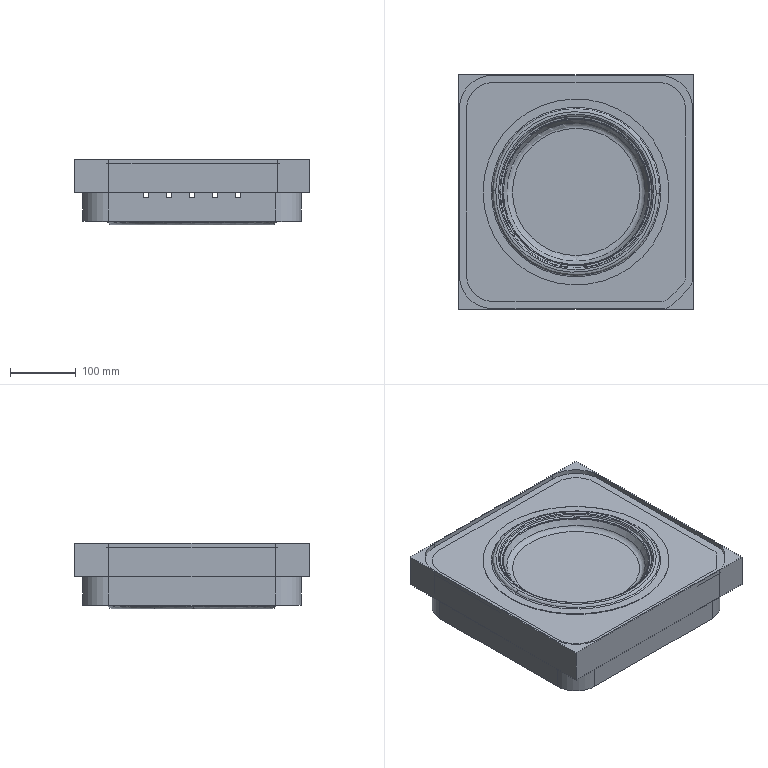NC program | NX | posted with a generic post | part box 356 x 356 x 99.5 mm
Lines 1 to 1240 of 165566:
N10 G17 G21 G94 G90
(01 , TOOL : D16R0.8)
N12 T00 M6
N14 G53
N16 G17 G0 G90 X-168.87 Y-27.35 S7000 M3 M8
N18 G43 Z200.5 H0
N20 Z51.5
N22 G94 G1 Y0. Z50.067 F4500.
N24 Y126.
N26 G2 X-126. Y168.87 R42.87
N28 G1 X126.
N30 G2 X168.87 Y126. R42.87
N32 G1 Y-129.787
N34 G2 X163.658 Y-142.401 R17.87
N36 G1 X163.609 Y-142.45
N38 X142.447 Y-163.612
N40 X142.398 Y-163.661
N42 G2 X129.787 Y-168.87 R17.87
N44 G1 X-126.
N46 G2 X-168.87 Y-126. R42.87
N48 G1 Y0.
N50 X-158.79
N52 Y126.
N54 G2 X-126. Y158.79 R32.79
N56 G1 X126.
N58 G2 X158.79 Y126. R32.79
N60 G1 Y-129.787
N62 G2 X156.48 Y-135.323 R7.79
N64 G1 X135.321 Y-156.482
N66 G2 X129.787 Y-158.79 R7.79
N68 G1 X-126.
N70 G2 X-158.79 Y-126. R32.79
N72 G1 Y0.
N74 X-148.71
N76 Y126.
N78 G2 X-126. Y148.71 R22.71
N80 G1 X126.
N82 G2 X148.71 Y126. R22.71
N84 G1 Y-128.838
N86 X128.838 Y-148.71
N88 X-126.
N90 G2 X-148.71 Y-126. R22.71
N92 G1 Y0.
N94 X-138.63
N96 Y126.
N98 G2 X-126. Y138.63 R12.63
N100 G1 X126.
N102 G2 X138.63 Y126. R12.63
N104 G1 Y-124.663
N106 X124.663 Y-138.63
N108 X-126.
N110 G2 X-138.63 Y-126. R12.63
N112 G1 Y0.
N114 X-128.55
N116 Y126.
N118 G2 X-126. Y128.55 R2.55
N120 G1 X126.
N122 G2 X128.55 Y126. R2.55
N124 G1 Y-120.488
N126 X120.488 Y-128.55
N128 X-126.
N130 G2 X-128.55 Y-126. R2.55
N132 G1 Y0.
N134 X-118.47
N136 Y118.47
N138 X118.47
N140 Y-116.312
N142 X116.312 Y-118.47
N144 X-118.47
N146 Y0.
N148 X-108.39
N150 Y108.39
N152 X108.39
N154 Y-108.39
N156 X-108.39
N158 Y0.
N160 X-98.31
N162 Y98.31
N164 X98.31
N166 Y-98.31
N168 X-98.31
N170 Y0.
N172 X-88.23
N174 Y88.23
N176 X88.23
N178 Y-88.23
N180 X-88.23
N182 Y0.
N184 X-78.15
N186 Y78.15
N188 X78.15
N190 Y-78.15
N192 X-78.15
N194 Y0.
N196 X-68.07
N198 Y68.07
N200 X68.07
N202 Y-68.07
N204 X-68.07
N206 Y0.
N208 X-57.99
N210 Y57.99
N212 X57.99
N214 Y-57.99
N216 X-57.99
N218 Y0.
N220 X-47.91
N222 Y47.91
N224 X47.91
N226 Y-47.91
N228 X-47.91
N230 Y0.
N232 X-37.83
N234 Y37.83
N236 X37.83
N238 Y-37.83
N240 X-37.83
N242 Y0.
N244 X-27.75
N246 Y27.75
N248 X27.75
N250 Y-27.75
N252 X-27.75
N254 Y0.
N256 X-17.67
N258 Y17.67
N260 X17.67
N262 Y-17.67
N264 X-17.67
N266 Y0.
N268 X-7.59
N270 Y7.59
N272 X7.59
N274 Y-7.59
N276 X-7.59
N278 Y0.
N280 X-0.39
N282 Y0.39
N284 X0.39
N286 Y-0.39
N288 X-0.39
N290 Y0.
N292 G3 X-3.59 Y3.2 R3.2
N294 G1 Z51.067
N296 G0 Z53.5
N298 X-168.8 Y-27.35
N300 Z51.067
N302 G1 Y0. Z49.633
N304 Y126.
N306 G2 X-126. Y168.8 R42.8
N308 G1 X126.
N310 G2 X168.8 Y126. R42.8
N312 G1 Y-129.787
N314 G2 X163.587 Y-142.373 R17.8
N316 G1 X142.373 Y-163.587
N318 G2 X129.787 Y-168.8 R17.8
N320 G1 X-126.
N322 G2 X-168.8 Y-126. R42.8
N324 G1 Y0.
N326 X-158.72
N328 Y126.
N330 G2 X-126. Y158.72 R32.72
N332 G1 X126.
N334 G2 X158.72 Y126. R32.72
N336 G1 Y-129.787
N338 G2 X156.459 Y-135.246 R7.72
N340 G1 X135.246 Y-156.459
N342 G2 X129.787 Y-158.72 R7.72
N344 G1 X-126.
N346 G2 X-158.72 Y-126. R32.72
N348 G1 Y0.
N350 X-148.64
N352 Y126.
N354 G2 X-126. Y148.64 R22.64
N356 G1 X126.
N358 G2 X148.64 Y126. R22.64
N360 G1 Y-128.809
N362 X128.809 Y-148.64
N364 X-126.
N366 G2 X-148.64 Y-126. R22.64
N368 G1 Y0.
N370 X-138.56
N372 Y126.
N374 G2 X-126. Y138.56 R12.56
N376 G1 X126.
N378 G2 X138.56 Y126. R12.56
N380 G1 Y-124.634
N382 X124.634 Y-138.56
N384 X-126.
N386 G2 X-138.56 Y-126. R12.56
N388 G1 Y0.
N390 X-128.48
N392 Y126.
N394 G2 X-126. Y128.48 R2.48
N396 G1 X126.
N398 G2 X128.48 Y126. R2.48
N400 G1 Y-120.459
N402 X120.459 Y-128.48
N404 X-126.
N406 G2 X-128.48 Y-126. R2.48
N408 G1 Y0.
N410 X-118.4
N412 Y118.4
N414 X118.4
N416 Y-116.283
N418 X116.283 Y-118.4
N420 X-118.4
N422 Y0.
N424 X-108.32
N426 Y108.32
N428 X108.32
N430 Y-108.32
N432 X-108.32
N434 Y0.
N436 X-98.24
N438 Y98.24
N440 X98.24
N442 Y-98.24
N444 X-98.24
N446 Y0.
N448 X-88.16
N450 Y88.16
N452 X88.16
N454 Y-88.16
N456 X-88.16
N458 Y0.
N460 X-78.08
N462 Y78.08
N464 X78.08
N466 Y-78.08
N468 X-78.08
N470 Y0.
N472 X-68.
N474 Y68.
N476 X68.
N478 Y-68.
N480 X-68.
N482 Y0.
N484 X-57.92
N486 Y57.92
N488 X57.92
N490 Y-57.92
N492 X-57.92
N494 Y0.
N496 X-47.84
N498 Y47.84
N500 X47.84
N502 Y-47.84
N504 X-47.84
N506 Y0.
N508 X-37.76
N510 Y37.76
N512 X37.76
N514 Y-37.76
N516 X-37.76
N518 Y0.
N520 X-27.68
N522 Y27.68
N524 X27.68
N526 Y-27.68
N528 X-27.68
N530 Y0.
N532 X-17.6
N534 Y17.6
N536 X17.6
N538 Y-17.6
N540 X-17.6
N542 Y0.
N544 X-7.52
N546 Y7.52
N548 X7.52
N550 Y-7.52
N552 X-7.52
N554 Y0.
N556 X-0.32
N558 Y0.32
N560 X0.32
N562 Y-0.32
N564 X-0.32
N566 Y0.
N568 G3 X-3.52 Y3.2 R3.2
N570 G1 Z50.633
N572 G0 Z53.067
N574 X-168.8 Y-27.35
N576 Z50.633
N578 G1 Y0. Z49.2
N580 Y126.
N582 G2 X-126. Y168.8 R42.8
N584 G1 X126.
N586 G2 X168.8 Y126. R42.8
N588 G1 Y-129.787
N590 G2 X163.587 Y-142.373 R17.8
N592 G1 X142.373 Y-163.587
N594 G2 X129.787 Y-168.8 R17.8
N596 G1 X-126.
N598 G2 X-168.8 Y-126. R42.8
N600 G1 Y0.
N602 X-158.72
N604 Y126.
N606 G2 X-126. Y158.72 R32.72
N608 G1 X126.
N610 G2 X158.72 Y126. R32.72
N612 G1 Y-129.787
N614 G2 X156.459 Y-135.246 R7.72
N616 G1 X135.246 Y-156.459
N618 G2 X129.787 Y-158.72 R7.72
N620 G1 X-126.
N622 G2 X-158.72 Y-126. R32.72
N624 G1 Y0.
N626 X-148.64
N628 Y126.
N630 G2 X-126. Y148.64 R22.64
N632 G1 X126.
N634 G2 X148.64 Y126. R22.64
N636 G1 Y-128.809
N638 X128.809 Y-148.64
N640 X-126.
N642 G2 X-148.64 Y-126. R22.64
N644 G1 Y0.
N646 X-138.56
N648 Y126.
N650 G2 X-126. Y138.56 R12.56
N652 G1 X126.
N654 G2 X138.56 Y126. R12.56
N656 G1 Y-124.634
N658 X124.634 Y-138.56
N660 X-126.
N662 G2 X-138.56 Y-126. R12.56
N664 G1 Y0.
N666 X-128.48
N668 Y126.
N670 G2 X-126. Y128.48 R2.48
N672 G1 X126.
N674 G2 X128.48 Y126. R2.48
N676 G1 Y-120.459
N678 X120.459 Y-128.48
N680 X-126.
N682 G2 X-128.48 Y-126. R2.48
N684 G1 Y0.
N686 X-118.4
N688 Y118.4
N690 X118.4
N692 Y-116.283
N694 X116.283 Y-118.4
N696 X-118.4
N698 Y0.
N700 X-108.32
N702 Y108.32
N704 X108.32
N706 Y-108.32
N708 X-108.32
N710 Y0.
N712 X-98.24
N714 Y98.24
N716 X98.24
N718 Y-98.24
N720 X-98.24
N722 Y0.
N724 X-88.16
N726 Y88.16
N728 X88.16
N730 Y-88.16
N732 X-88.16
N734 Y0.
N736 X-78.08
N738 Y78.08
N740 X78.08
N742 Y-78.08
N744 X-78.08
N746 Y0.
N748 X-68.
N750 Y68.
N752 X68.
N754 Y-68.
N756 X-68.
N758 Y0.
N760 X-57.92
N762 Y57.92
N764 X57.92
N766 Y-57.92
N768 X-57.92
N770 Y0.
N772 X-47.84
N774 Y47.84
N776 X47.84
N778 Y-47.84
N780 X-47.84
N782 Y0.
N784 X-37.76
N786 Y37.76
N788 X37.76
N790 Y-37.76
N792 X-37.76
N794 Y0.
N796 X-27.68
N798 Y27.68
N800 X27.68
N802 Y-27.68
N804 X-27.68
N806 Y0.
N808 X-17.6
N810 Y17.6
N812 X17.6
N814 Y-17.6
N816 X-17.6
N818 Y0.
N820 X-7.52
N822 Y7.52
N824 X7.52
N826 Y-7.52
N828 X-7.52
N830 Y0.
N832 X-0.32
N834 Y0.32
N836 X0.32
N838 Y-0.32
N840 X-0.32
N842 Y0.
N844 G3 X-3.52 Y3.2 R3.2
N846 G1 Z50.2
N848 G0 Z52.633
N850 X-168.8 Y-27.238
N852 Z50.2
N854 G1 Y0. Z48.773
N856 Y126.
N858 G2 X-126. Y168.8 R42.8
N860 G1 X126.
N862 G2 X168.8 Y126. R42.8
N864 G1 Y-129.787
N866 G2 X163.587 Y-142.373 R17.8
N868 G1 X142.373 Y-163.587
N870 G2 X129.787 Y-168.8 R17.8
N872 G1 X-126.
N874 G2 X-168.8 Y-126. R42.8
N876 G1 Y0.
N878 X-158.72
N880 Y126.
N882 G2 X-126. Y158.72 R32.72
N884 G1 X126.
N886 G2 X158.72 Y126. R32.72
N888 G1 Y-129.787
N890 G2 X156.459 Y-135.246 R7.72
N892 G1 X135.246 Y-156.459
N894 G2 X129.787 Y-158.72 R7.72
N896 G1 X-126.
N898 G2 X-158.72 Y-126. R32.72
N900 G1 Y0.
N902 X-148.64
N904 Y126.
N906 G2 X-126. Y148.64 R22.64
N908 G1 X126.
N910 G2 X148.64 Y126. R22.64
N912 G1 Y-128.809
N914 X128.809 Y-148.64
N916 X-126.
N918 G2 X-148.64 Y-126. R22.64
N920 G1 Y0.
N922 X-138.56
N924 Y126.
N926 G2 X-126. Y138.56 R12.56
N928 G1 X-34.777
N930 Y128.48
N932 G3 X-128.48 Y34.777 R133.104
N934 G1 X-130.973 Y25.849
N936 X-128.48 Y34.777
N938 Y126.
N940 G2 X-126. Y128.48 R2.48
N942 G1 X-118.4
N944 Y118.4
N946 X-80.517
N948 X-72.605 Y120.717
N950 X-80.517 Y118.4
N952 G3 X-118.4 Y80.517 R143.184
N954 G1 X-120.717 Y72.605
N956 X-118.4 Y80.517
N958 Y118.4
N960 X-111.2 Y111.2
N962 X-101.241
N964 G3 X-111.2 Y101.241 R150.384
N966 G1 Y111.2
N968 X-118.4 Y118.4
N970 Y128.48
N972 X-34.777
N974 X-25.849 Y130.973
N976 X-34.777 Y128.48
N978 Y138.56
N980 X126.
N982 G2 X138.56 Y126. R12.56
N984 G1 Y34.777
N986 X128.48
N988 G3 X34.777 Y128.48 R133.104
N990 G1 X25.849 Y130.973
N992 X34.777 Y128.48
N994 X126.
N996 G2 X128.48 Y126. R2.48
N998 G1 Y80.517
N1000 X118.4
N1002 G3 X80.517 Y118.4 R143.184
N1004 G1 X72.605 Y120.717
N1006 X80.517 Y118.4
N1008 X118.4
N1010 Y80.517
N1012 X120.717 Y72.605
N1014 X118.4 Y80.517
N1016 X111.2 Y101.241
N1018 G3 X101.241 Y111.2 R150.384
N1020 G1 X111.2
N1022 Y101.241
N1024 X118.4 Y80.517
N1026 X128.48
N1028 Y34.777
N1030 X130.973 Y25.849
N1032 X128.48 Y34.777
N1034 X138.56
N1036 Y-124.634
N1038 X124.634 Y-138.56
N1040 X34.777
N1042 Y-128.48
N1044 G3 X128.48 Y-34.777 R133.104
N1046 G1 X130.973 Y-25.849
N1048 X128.48 Y-34.777
N1050 Y-120.459
N1052 X120.459 Y-128.48
N1054 X34.777
N1056 X25.849 Y-130.973
N1058 X34.777 Y-128.48
N1060 X80.517 Y-118.4
N1062 G3 X118.4 Y-80.517 R143.184
N1064 G1 X120.717 Y-72.605
N1066 X118.4 Y-80.517
N1068 Y-116.283
N1070 X116.283 Y-118.4
N1072 X111.2
N1074 Y-111.2
N1076 X101.241
N1078 G3 X111.2 Y-101.241 R150.384
N1080 G1 Y-111.2
N1082 Y-118.4
N1084 X80.517
N1086 X34.777 Y-128.48
N1088 Y-138.56
N1090 X-126.
N1092 G2 X-138.56 Y-126. R12.56
N1094 G1 Y-34.777
N1096 X-128.48
N1098 G3 X-34.777 Y-128.48 R133.104
N1100 G1 X-25.849 Y-130.973
N1102 X-34.777 Y-128.48
N1104 X-34.251 Y-126.534
N1106 G2 X-126.534 Y34.251 R131.088
N1108 X-34.251 Y-126.534 R-131.088
N1110 G1 X-34.777 Y-128.48
N1112 X-126.
N1114 G2 X-128.48 Y-126. R2.48
N1116 G1 Y-118.4
N1118 X-118.4
N1120 Y-80.517
N1122 X-120.717 Y-72.605
N1124 X-118.4 Y-80.517
N1126 G3 X-80.517 Y-118.4 R143.184
N1128 G1 X-72.605 Y-120.717
N1130 X-80.517 Y-118.4
N1132 X-118.4
N1134 X-111.2 Y-111.2
N1136 Y-101.241
N1138 G3 X-101.241 Y-111.2 R150.384
N1140 G1 X-111.2
N1142 X-118.4 Y-118.4
N1144 X-128.48
N1146 Y-34.777
N1148 X-130.973 Y-25.849
N1150 X-128.48 Y-34.777
N1152 X-138.56
N1154 Y0.
N1156 G3 X-141.76 Y3.2 R3.2
N1158 G1 Z49.773
N1160 G0 Z52.2
N1162 X-168.8 Y-27.238
N1164 Z49.773
N1166 G1 Y0. Z48.345
N1168 Y126.
N1170 G2 X-126. Y168.8 R42.8
N1172 G1 X126.
N1174 G2 X168.8 Y126. R42.8
N1176 G1 Y-129.787
N1178 G2 X163.587 Y-142.373 R17.8
N1180 G1 X142.373 Y-163.587
N1182 G2 X129.787 Y-168.8 R17.8
N1184 G1 X-126.
N1186 G2 X-168.8 Y-126. R42.8
N1188 G1 Y0.
N1190 X-158.72
N1192 Y126.
N1194 G2 X-126. Y158.72 R32.72
N1196 G1 X126.
N1198 G2 X158.72 Y126. R32.72
N1200 G1 Y-129.787
N1202 G2 X156.459 Y-135.246 R7.72
N1204 G1 X135.246 Y-156.459
N1206 G2 X129.787 Y-158.72 R7.72
N1208 G1 X-126.
N1210 G2 X-158.72 Y-126. R32.72
N1212 G1 Y0.
N1214 X-148.64
N1216 Y126.
N1218 G2 X-126. Y148.64 R22.64
N1220 G1 X126.
N1222 G2 X148.64 Y126. R22.64
N1224 G1 Y-128.809
N1226 X128.809 Y-148.64
N1228 X-126.
N1230 G2 X-148.64 Y-126. R22.64
N1232 G1 Y0.
N1234 X-138.56
N1236 Y126.
N1238 G2 X-126. Y138.56 R12.56
N1240 G1 X-38.012
N1242 Y128.48
N1244 G3 X-128.48 Y38.012 R133.985
N1246 G1 X-131.024 Y29.635
N1248 X-128.48 Y38.012
N1250 Y126.
N1252 G2 X-126. Y128.48 R2.48
N1254 G1 X-118.4
N1256 Y118.4
N1258 X-82.074
N1260 X-74.227 Y120.738
N1262 X-82.074 Y118.4
N1264 G3 X-118.4 Y82.074 R144.065
N1266 G1 X-120.738 Y74.227
N1268 X-118.4 Y82.074
N1270 Y118.4
N1272 X-111.2 Y111.2
N1274 X-102.546
N1276 G3 X-111.2 Y102.546 R151.265
N1278 G1 Y111.2
N1280 X-118.4 Y118.4
N1282 Y128.48
N1284 X-38.012
N1286 X-29.635 Y131.024
N1288 X-38.012 Y128.48
N1290 Y138.56
N1292 X126.
N1294 G2 X138.56 Y126. R12.56
N1296 G1 Y38.012
N1298 X128.48
N1300 G3 X38.012 Y128.48 R133.985
N1302 G1 X29.635 Y131.024
N1304 X38.012 Y128.48
N1306 X126.
N1308 G2 X128.48 Y126. R2.48
N1310 G1 Y118.4
N1312 X118.4
N1314 Y82.074
N1316 X120.738 Y74.227
N1318 X118.4 Y82.074
N1320 G3 X82.074 Y118.4 R144.065
N1322 G1 X74.227 Y120.738
N1324 X82.074 Y118.4
N1326 X118.4
N1328 X111.2 Y111.2
N1330 Y102.546
N1332 G3 X102.546 Y111.2 R151.265
N1334 G1 X111.2
N1336 X118.4 Y118.4
N1338 X128.48
N1340 Y38.012
N1342 X131.024 Y29.635
N1344 X128.48 Y38.012
N1346 X138.56
N1348 Y-124.634
N1350 X124.634 Y-138.56
N1352 X38.012
N1354 Y-128.48
N1356 G3 X128.48 Y-38.012 R133.985
N1358 G1 X131.024 Y-29.635
N1360 X128.48 Y-38.012
N1362 Y-120.459
N1364 X120.459 Y-128.48
N1366 X38.012
N1368 X29.635 Y-131.024
N1370 X38.012 Y-128.48
N1372 X82.074 Y-118.4
N1374 G3 X118.4 Y-82.074 R144.065
N1376 G1 X120.738 Y-74.227
N1378 X118.4 Y-82.074
N1380 Y-116.283
N1382 X116.283 Y-118.4
N1384 X111.2
N1386 Y-111.2
N1388 X102.546
N1390 G3 X111.2 Y-102.546 R151.265
N1392 G1 Y-111.2
N1394 Y-118.4
N1396 X82.074
N1398 X38.012 Y-128.48
N1400 Y-138.56
N1402 X-126.
N1404 G2 X-138.56 Y-126. R12.56
N1406 G1 Y-38.012
N1408 X-128.48
N1410 G3 X-38.012 Y-128.48 R133.985
N1412 G1 X-29.635 Y-131.024
N1414 X-38.012 Y-128.48
N1416 X-37.44 Y-126.547
N1418 G2 X-126.547 Y37.44 R131.969
N1420 X-37.44 Y-126.547 R-131.969
N1422 G1 X-38.012 Y-128.48
N1424 X-126.
N1426 G2 X-128.48 Y-126. R2.48
N1428 G1 Y-118.4
N1430 X-118.4
N1432 Y-82.074
N1434 X-120.738 Y-74.227
N1436 X-118.4 Y-82.074
N1438 G3 X-82.074 Y-118.4 R144.065
N1440 G1 X-74.227 Y-120.738
N1442 X-82.074 Y-118.4
N1444 X-118.4
N1446 X-111.2 Y-111.2
N1448 Y-102.546
N1450 G3 X-102.546 Y-111.2 R151.265
N1452 G1 X-111.2
N1454 X-118.4 Y-118.4
N1456 X-128.48
N1458 Y-38.012
N1460 X-131.024 Y-29.635
N1462 X-128.48 Y-38.012
N1464 X-138.56
N1466 Y0.
N1468 G3 X-141.76 Y3.2 R3.2
N1470 G1 Z49.345
N1472 G0 Z51.773
N1474 X-168.8 Y-27.238
N1476 Z49.345
N1478 G1 Y0. Z47.918
N1480 Y126.
N1482 G2 X-126. Y168.8 R42.8
N1484 G1 X126.
N1486 G2 X168.8 Y126. R42.8
N1488 G1 Y-129.787
N1490 G2 X163.587 Y-142.373 R17.8
N1492 G1 X142.373 Y-163.587
N1494 G2 X129.787 Y-168.8 R17.8
N1496 G1 X-126.
N1498 G2 X-168.8 Y-126. R42.8
N1500 G1 Y0.
N1502 X-158.72
N1504 Y126.
N1506 G2 X-126. Y158.72 R32.72
N1508 G1 X126.
N1510 G2 X158.72 Y126. R32.72
N1512 G1 Y-129.787
N1514 G2 X156.459 Y-135.246 R7.72
N1516 G1 X135.246 Y-156.459
N1518 G2 X129.787 Y-158.72 R7.72
N1520 G1 X-126.
N1522 G2 X-158.72 Y-126. R32.72
N1524 G1 Y0.
N1526 X-148.64
N1528 Y126.
N1530 G2 X-126. Y148.64 R22.64
N1532 G1 X126.
N1534 G2 X148.64 Y126. R22.64
N1536 G1 Y-128.809
N1538 X128.809 Y-148.64
N1540 X-126.
N1542 G2 X-148.64 Y-126. R22.64
N1544 G1 Y0.
N1546 X-138.56
N1548 Y126.
N1550 G2 X-126. Y138.56 R12.56
N1552 G1 X-40.122
N1554 Y128.48
N1556 G3 X-128.48 Y40.128 R134.602
N1558 G1 X-131.058 Y32.037
N1560 X-128.48 Y40.128
N1562 Y126.
N1564 G2 X-126. Y128.48 R2.48
N1566 G1 X-118.4
N1568 Y118.4
N1570 X-83.148
N1572 X-75.344 Y120.752
N1574 X-83.148 Y118.4
N1576 G3 X-118.4 Y83.149 R144.682
N1578 G1 X-120.752 Y75.345
N1580 X-118.4 Y83.149
N1582 Y118.4
N1584 X-111.2 Y111.2
N1586 X-103.45
N1588 G3 X-111.2 Y103.45 R151.882
N1590 G1 Y111.2
N1592 X-118.4 Y118.4
N1594 Y128.48
N1596 X-40.122
N1598 X-32.03 Y131.058
N1600 X-40.122 Y128.48
N1602 Y138.56
N1604 X126.
N1606 G2 X138.56 Y126. R12.56
N1608 G1 Y40.129
N1610 X128.48
N1612 G3 X40.122 Y128.48 R134.602
N1614 G1 X32.03 Y131.058
N1616 X40.122 Y128.48
N1618 X126.
N1620 G2 X128.48 Y126. R2.48
N1622 G1 Y118.4
N1624 X118.4
N1626 Y83.149
N1628 X120.752 Y75.346
N1630 X118.4 Y83.149
N1632 G3 X83.148 Y118.4 R144.682
N1634 G1 X75.344 Y120.752
N1636 X83.148 Y118.4
N1638 X118.4
N1640 X111.2 Y111.2
N1642 Y103.451
N1644 G3 X103.451 Y111.2 R151.882
N1646 G1 X111.2
N1648 X118.4 Y118.4
N1650 X128.48
N1652 Y40.129
N1654 X131.058 Y32.039
N1656 X128.48 Y40.129
N1658 X138.56
N1660 Y-124.634
N1662 X124.634 Y-138.56
N1664 X40.142
N1666 Y-128.48
N1668 G3 X128.48 Y-40.136 R134.602
N1670 G1 X131.058 Y-32.045
N1672 X128.48 Y-40.136
N1674 Y-83.156
N1676 X118.4
N1678 Y-116.283
N1680 X116.283 Y-118.4
N1682 X111.2
N1684 Y-111.2
N1686 X103.457
N1688 G3 X111.2 Y-103.457 R151.882
N1690 G1 Y-111.2
N1692 Y-118.4
N1694 X83.157
N1696 X75.353 Y-120.752
N1698 X83.157 Y-118.4
N1700 G3 X118.4 Y-83.156 R144.682
N1702 G1 X120.752 Y-75.352
N1704 X118.4 Y-83.156
N1706 X128.48
N1708 Y-120.459
N1710 X120.459 Y-128.48
N1712 X40.142
N1714 X32.053 Y-131.058
N1716 X40.142 Y-128.48
N1718 Y-138.56
N1720 X-126.
N1722 G2 X-138.56 Y-126. R12.56
N1724 G1 Y-40.134
N1726 X-128.48
N1728 G3 X-40.141 Y-128.48 R134.602
N1730 G1 X-32.052 Y-131.058
N1732 X-40.141 Y-128.48
N1734 X-39.54 Y-126.556
N1736 G2 X-126.552 Y39.537 R132.586
N1738 X-39.54 Y-126.556 R-132.586
N1740 G1 X-40.141 Y-128.48
N1742 X-126.
N1744 G2 X-128.48 Y-126. R2.48
N1746 G1 Y-83.155
N1748 X-118.4
N1750 G3 X-83.156 Y-118.4 R144.682
N1752 G1 X-75.353 Y-120.752
N1754 X-83.156 Y-118.4
N1756 X-118.4
N1758 Y-83.155
N1760 X-120.752 Y-75.351
N1762 X-118.4 Y-83.155
N1764 X-111.2 Y-103.457
N1766 G3 X-103.457 Y-111.2 R151.882
N1768 G1 X-111.2
N1770 Y-103.457
N1772 X-118.4 Y-83.155
N1774 X-128.48
N1776 Y-40.134
N1778 X-131.058 Y-32.044
N1780 X-128.48 Y-40.134
N1782 X-138.56
N1784 Y0.
N1786 G3 X-141.76 Y3.2 R3.2
N1788 G1 Z48.918
N1790 G0 Z51.345
N1792 X-168.8 Y-27.238
N1794 Z48.918
N1796 G1 Y0. Z47.49
N1798 Y126.
N1800 G2 X-126. Y168.8 R42.8
N1802 G1 X126.
N1804 G2 X168.8 Y126. R42.8
N1806 G1 Y-129.787
N1808 G2 X163.587 Y-142.373 R17.8
N1810 G1 X142.373 Y-163.587
N1812 G2 X129.787 Y-168.8 R17.8
N1814 G1 X-126.
N1816 G2 X-168.8 Y-126. R42.8
N1818 G1 Y0.
N1820 X-158.72
N1822 Y126.
N1824 G2 X-126. Y158.72 R32.72
N1826 G1 X126.
N1828 G2 X158.72 Y126. R32.72
N1830 G1 Y-129.787
N1832 G2 X156.459 Y-135.246 R7.72
N1834 G1 X135.246 Y-156.459
N1836 G2 X129.787 Y-158.72 R7.72
N1838 G1 X-126.
N1840 G2 X-158.72 Y-126. R32.72
N1842 G1 Y0.
N1844 X-148.64
N1846 Y126.
N1848 G2 X-126. Y148.64 R22.64
N1850 G1 X126.
N1852 G2 X148.64 Y126. R22.64
N1854 G1 Y-128.809
N1856 X128.809 Y-148.64
N1858 X-126.
N1860 G2 X-148.64 Y-126. R22.64
N1862 G1 Y0.
N1864 X-138.56
N1866 Y126.
N1868 G2 X-126. Y138.56 R12.56
N1870 G1 X-41.747
N1872 Y128.48
N1874 G3 X-128.48 Y41.746 R135.09
N1876 G1 X-131.084 Y33.845
N1878 X-128.48 Y41.746
N1880 Y126.
N1882 G2 X-126. Y128.48 R2.48
N1884 G1 X-118.4
N1886 Y118.4
N1888 X-84.003
N1890 X-76.232 Y120.764
N1892 X-84.003 Y118.4
N1894 G3 X-118.4 Y84.003 R145.17
N1896 G1 X-120.764 Y76.232
N1898 X-118.4 Y84.003
N1900 Y118.4
N1902 X-111.2 Y111.2
N1904 X-104.173
N1906 G3 X-111.2 Y104.173 R152.37
N1908 G1 Y111.2
N1910 X-118.4 Y118.4
N1912 Y128.48
N1914 X-41.747
N1916 X-33.846 Y131.084
N1918 X-41.747 Y128.48
N1920 Y138.56
N1922 X126.
N1924 G2 X138.56 Y126. R12.56
N1926 G1 Y41.735
N1928 X128.48
N1930 G3 X41.743 Y128.48 R135.09
N1932 G1 X33.843 Y131.084
N1934 X41.743 Y128.48
N1936 X126.
N1938 G2 X128.48 Y126. R2.48
N1940 G1 Y118.4
N1942 X118.4
N1944 Y83.998
N1946 X120.763 Y76.227
N1948 X118.4 Y83.998
N1950 G3 X83.999 Y118.4 R145.17
N1952 G1 X76.229 Y120.764
N1954 X83.999 Y118.4
N1956 X118.4
N1958 X111.2 Y111.2
N1960 Y104.169
N1962 G3 X104.169 Y111.2 R152.37
N1964 G1 X111.2
N1966 X118.4 Y118.4
N1968 X128.48
N1970 Y41.735
N1972 X131.083 Y33.833
N1974 X128.48 Y41.735
N1976 X138.56
N1978 Y-124.634
N1980 X124.634 Y-138.56
N1982 X41.731
N1984 Y-128.48
N1986 G3 X128.48 Y-41.731 R135.09
N1988 G1 X131.083 Y-33.829
N1990 X128.48 Y-41.731
N1992 Y-83.994
N1994 X118.4
N1996 Y-116.283
N1998 X116.283 Y-118.4
N2000 X111.2
N2002 Y-111.2
N2004 X104.165
N2006 G3 X111.2 Y-104.165 R152.37
N2008 G1 Y-111.2
N2010 Y-118.4
N2012 X83.994
N2014 X76.223 Y-120.763
N2016 X83.994 Y-118.4
N2018 G3 X118.4 Y-83.994 R145.17
N2020 G1 X120.763 Y-76.223
N2022 X118.4 Y-83.994
N2024 X128.48
N2026 Y-120.459
N2028 X120.459 Y-128.48
N2030 X41.731
N2032 X33.828 Y-131.083
N2034 X41.731 Y-128.48
N2036 Y-138.56
N2038 X-126.
N2040 G2 X-138.56 Y-126. R12.56
N2042 G1 Y-41.742
N2044 X-128.48
N2046 G3 X-41.734 Y-128.48 R135.09
N2048 G1 X-33.832 Y-131.083
N2050 X-41.734 Y-128.48
N2052 X-41.112 Y-126.563
N2054 G2 X-126.566 Y41.112 R133.074
N2056 X-41.112 Y-126.563 R-133.074
N2058 G1 X-41.734 Y-128.48
N2060 X-126.
N2062 G2 X-128.48 Y-126. R2.48
N2064 G1 Y-118.4
N2066 X-118.4
N2068 Y-83.999
N2070 X-120.764 Y-76.228
N2072 X-118.4 Y-83.999
N2074 G3 X-83.997 Y-118.4 R145.17
N2076 G1 X-76.226 Y-120.763
N2078 X-83.997 Y-118.4
N2080 X-118.4
N2082 X-111.2 Y-111.2
N2084 Y-104.168
N2086 G3 X-104.168 Y-111.2 R152.37
N2088 G1 X-111.2
N2090 X-118.4 Y-118.4
N2092 X-128.48
N2094 Y-41.742
N2096 X-131.084 Y-33.841
N2098 X-128.48 Y-41.742
N2100 X-138.56
N2102 Y0.
N2104 G3 X-141.76 Y3.2 R3.2
N2106 G1 Z48.49
N2108 G0 Z50.918
N2110 X-168.8 Y-27.238
N2112 Z48.49
N2114 G1 Y0. Z47.063
N2116 Y126.
N2118 G2 X-126. Y168.8 R42.8
N2120 G1 X126.
N2122 G2 X168.8 Y126. R42.8
N2124 G1 Y-129.787
N2126 G2 X163.587 Y-142.373 R17.8
N2128 G1 X142.373 Y-163.587
N2130 G2 X129.787 Y-168.8 R17.8
N2132 G1 X-126.
N2134 G2 X-168.8 Y-126. R42.8
N2136 G1 Y0.
N2138 X-158.72
N2140 Y126.
N2142 G2 X-126. Y158.72 R32.72
N2144 G1 X126.
N2146 G2 X158.72 Y126. R32.72
N2148 G1 Y-129.787
N2150 G2 X156.459 Y-135.246 R7.72
N2152 G1 X135.246 Y-156.459
N2154 G2 X129.787 Y-158.72 R7.72
N2156 G1 X-126.
N2158 G2 X-158.72 Y-126. R32.72
N2160 G1 Y0.
N2162 X-148.64
N2164 Y126.
N2166 G2 X-126. Y148.64 R22.64
N2168 G1 X126.
N2170 G2 X148.64 Y126. R22.64
N2172 G1 Y-128.809
N2174 X128.809 Y-148.64
N2176 X-126.
N2178 G2 X-148.64 Y-126. R22.64
N2180 G1 Y0.
N2182 X-138.56
N2184 Y126.
N2186 G2 X-126. Y138.56 R12.56
N2188 G1 X-43.027
N2190 Y128.48
N2192 G3 X-128.48 Y43.05 R135.507
N2194 G1 X-131.104 Y35.289
N2196 X-128.48 Y43.05
N2198 Y126.
N2200 G2 X-126. Y128.48 R2.48
N2202 G1 X-118.4
N2204 Y118.4
N2206 X-84.696
N2208 X-76.952 Y120.773
N2210 X-84.696 Y118.4
N2212 G3 X-118.4 Y84.701 R145.587
N2214 G1 X-120.773 Y76.957
N2216 X-118.4 Y84.701
N2218 Y118.4
N2220 X-111.2 Y111.2
N2222 X-104.761
N2224 G3 X-111.2 Y104.762 R152.787
N2226 G1 Y111.2
N2228 X-118.4 Y118.4
N2230 Y128.48
N2232 X-43.027
N2234 X-35.263 Y131.104
N2236 X-43.027 Y128.48
N2238 Y138.56
N2240 X126.
N2242 G2 X138.56 Y126. R12.56
N2244 G1 Y43.02
N2246 X128.48
N2248 G3 X54.076 Y124.237 R135.495
N2250 X43.032 Y128.48 R135.507
N2252 G1 X35.268 Y131.104
N2254 X43.032 Y128.48
N2256 X126.
N2258 G2 X128.48 Y126. R2.48
N2260 G1 Y118.4
N2262 X118.4
N2264 Y84.692
N2266 X120.773 Y76.948
N2268 X118.4 Y84.692
N2270 G3 X84.695 Y118.4 R145.575
N2272 G1 X76.952 Y120.773
N2274 X84.695 Y118.4
N2276 X118.4
N2278 X111.2 Y111.2
N2280 Y104.758
N2282 G3 X104.758 Y111.2 R152.775
N2284 G1 X111.2
N2286 X118.4 Y118.4
N2288 X128.48
N2290 Y43.02
N2292 X131.104 Y35.254
N2294 X128.48 Y43.02
N2296 X138.56
N2298 Y-124.634
N2300 X124.634 Y-138.56
N2302 X43.02
N2304 Y-128.48
N2306 G3 X128.48 Y-43.014 R135.495
N2308 G1 X131.104 Y-35.249
N2310 X128.48 Y-43.014
N2312 Y-84.687
N2314 X118.4
N2316 Y-116.283
N2318 X116.283 Y-118.4
N2320 X111.2
N2322 Y-111.2
N2324 X104.753
N2326 G3 X111.2 Y-104.753 R152.775
N2328 G1 Y-111.2
N2330 Y-118.4
N2332 X84.688
N2334 X76.944 Y-120.773
N2336 X84.688 Y-118.4
N2338 G3 X118.4 Y-84.687 R145.575
N2340 G1 X120.773 Y-76.943
N2342 X118.4 Y-84.687
N2344 X128.48
N2346 Y-120.459
N2348 X120.459 Y-128.48
N2350 X43.02
N2352 X35.256 Y-131.104
N2354 X43.02 Y-128.48
N2356 Y-138.56
N2358 X-126.
N2360 G2 X-138.56 Y-126. R12.56
N2362 G1 Y-43.047
N2364 X-128.48
N2366 G3 X-43.031 Y-128.48 R135.495
N2368 G1 X-35.267 Y-131.104
N2370 X-43.031 Y-128.48
N2372 X-42.391 Y-126.568
N2374 G2 X-128.89 Y34.723 R133.479
N2376 X53.271 Y122.389 R133.491
N2378 X-42.391 Y-126.568 R133.479
N2380 G1 X-43.031 Y-128.48
N2382 X-126.
N2384 G2 X-128.48 Y-126. R2.48
N2386 G1 Y-118.4
N2388 X-118.4
N2390 Y-84.702
N2392 X-120.773 Y-76.959
N2394 X-118.4 Y-84.702
N2396 G3 X-84.699 Y-118.4 R145.575
N2398 G1 X-76.955 Y-120.773
N2400 X-84.699 Y-118.4
N2402 X-118.4
N2404 X-111.2 Y-111.2
N2406 Y-104.764
N2408 G3 X-104.764 Y-111.2 R152.775
N2410 G1 X-111.2
N2412 X-118.4 Y-118.4
N2414 X-128.48
N2416 Y-43.047
N2418 X-131.104 Y-35.286
N2420 X-128.48 Y-43.047
N2422 X-138.56
N2424 Y0.
N2426 G3 X-141.76 Y3.2 R3.2
N2428 G1 Z48.063
N2430 G0 Z50.49
N2432 X-168.8 Y-27.238
N2434 Z48.063
N2436 G1 Y0. Z46.635
N2438 Y126.
N2440 G2 X-126. Y168.8 R42.8
N2442 G1 X126.
N2444 G2 X168.8 Y126. R42.8
N2446 G1 Y-129.787
N2448 G2 X163.587 Y-142.373 R17.8
N2450 G1 X142.373 Y-163.587
N2452 G2 X129.787 Y-168.8 R17.8
N2454 G1 X-126.
N2456 G2 X-168.8 Y-126. R42.8
N2458 G1 Y0.
N2460 X-158.72
N2462 Y126.
N2464 G2 X-126. Y158.72 R32.72
N2466 G1 X126.
N2468 G2 X158.72 Y126. R32.72
N2470 G1 Y-129.787
N2472 G2 X156.459 Y-135.246 R7.72
N2474 G1 X135.246 Y-156.459
N2476 G2 X129.787 Y-158.72 R7.72
N2478 G1 X-126.